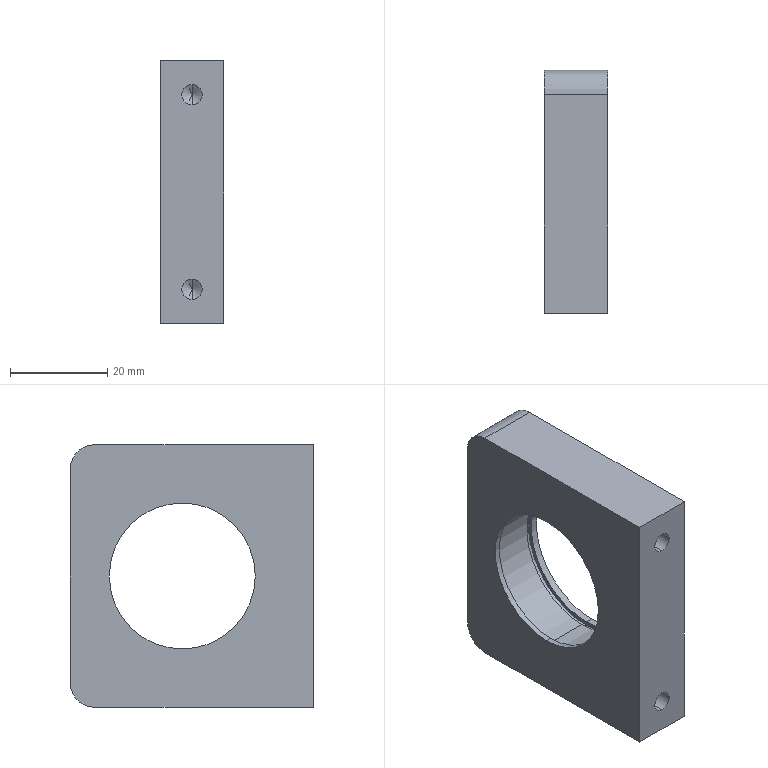Part | SolidWorks | features ICE 4, 3DProfileFeature 2, HoleWzd 2, ExtruThin 1, Fillet 1, RevCut 1 | 1 solid | 35 faces | box 13 x 50 x 54 mm | volume 23974 mm3 | cylinder 18 | plane 9 | cone 8 | commonest cylinder face diameters 3.3 x4 4.2 x4 32 x4 10 x2 30 x2 33.7 x2
STEP:
#1=CARTESIAN_POINT('',(-6.5,39.9,-16.65));
#2=VERTEX_POINT('',#1);
#3=CARTESIAN_POINT('',(-6.5,39.9,-13.35));
#4=VERTEX_POINT('',#3);
#5=CARTESIAN_POINT('',(-6.5,39.9,-15.));
#6=DIRECTION('',(0.,1.,0.));
#7=DIRECTION('',(0.,0.,1.));
#8=AXIS2_PLACEMENT_3D('',#5,#6,#7);
#9=CIRCLE('',#8,1.65);
#10=EDGE_CURVE('',#2,#4,#9,.T.);
#11=ORIENTED_EDGE('',*,*,#10,.F.);
#12=CARTESIAN_POINT('',(-6.5,50.,-16.65));
#13=VERTEX_POINT('',#12);
#14=CARTESIAN_POINT('',(-6.5,50.,-16.65));
#15=DIRECTION('',(0.,1.,0.));
#16=VECTOR('',#15,1000.);
#17=LINE('',#14,#16);
#18=EDGE_CURVE('',#2,#13,#17,.T.);
#19=ORIENTED_EDGE('',*,*,#18,.T.);
#20=CARTESIAN_POINT('',(-6.5,50.,-13.35));
#21=VERTEX_POINT('',#20);
#22=CARTESIAN_POINT('',(-6.5,50.,-15.));
#23=DIRECTION('',(0.,1.,0.));
#24=DIRECTION('',(0.,0.,1.));
#25=AXIS2_PLACEMENT_3D('',#22,#23,#24);
#26=CIRCLE('',#25,1.65);
#27=EDGE_CURVE('',#13,#21,#26,.T.);
#28=ORIENTED_EDGE('',*,*,#27,.T.);
#29=CARTESIAN_POINT('',(-6.5,50.,-13.35));
#30=DIRECTION('',(0.,1.,0.));
#31=VECTOR('',#30,1000.);
#32=LINE('',#29,#31);
#33=EDGE_CURVE('',#4,#21,#32,.T.);
#34=ORIENTED_EDGE('',*,*,#33,.F.);
#35=EDGE_LOOP('',(#11,#19,#28,#34));
#36=FACE_OUTER_BOUND('',#35,.T.);
#37=CARTESIAN_POINT('',(-6.5,50.,-15.));
#38=DIRECTION('',(0.,1.,0.));
#39=DIRECTION('',(0.,0.,1.));
#40=AXIS2_PLACEMENT_3D('',#37,#38,#39);
#41=CYLINDRICAL_SURFACE('',#40,1.65);
#42=ADVANCED_FACE('',(#36),#41,.F.);
#43=CARTESIAN_POINT('',(-6.5,38.909,-15.));
#44=VERTEX_POINT('',#43);
#45=CARTESIAN_POINT('',(-6.5,39.9,-13.35));
#46=DIRECTION('',(0.,0.515,0.8572));
#47=VECTOR('',#46,1000.);
#48=LINE('',#45,#47);
#49=EDGE_CURVE('',#44,#4,#48,.T.);
#50=ORIENTED_EDGE('',*,*,#49,.F.);
#51=CARTESIAN_POINT('',(-6.5,39.9,-16.65));
#52=DIRECTION('',(0.,0.515,-0.8572));
#53=VECTOR('',#52,1000.);
#54=LINE('',#51,#53);
#55=EDGE_CURVE('',#44,#2,#54,.T.);
#56=ORIENTED_EDGE('',*,*,#55,.T.);
#57=ORIENTED_EDGE('',*,*,#10,.T.);
#58=EDGE_LOOP('',(#50,#56,#57));
#59=FACE_OUTER_BOUND('',#58,.T.);
#60=CARTESIAN_POINT('',(-6.5,39.9,-15.));
#61=DIRECTION('',(0.,1.,0.));
#62=DIRECTION('',(0.,0.,1.));
#63=AXIS2_PLACEMENT_3D('',#60,#61,#62);
#64=CONICAL_SURFACE('',#63,1.65,1.03);
#65=ADVANCED_FACE('',(#59),#64,.F.);
#66=CARTESIAN_POINT('',(-6.5,39.9,13.35));
#67=VERTEX_POINT('',#66);
#68=CARTESIAN_POINT('',(-6.5,39.9,16.65));
#69=VERTEX_POINT('',#68);
#70=CARTESIAN_POINT('',(-6.5,39.9,15.));
#71=DIRECTION('',(0.,1.,0.));
#72=DIRECTION('',(0.,0.,1.));
#73=AXIS2_PLACEMENT_3D('',#70,#71,#72);
#74=CIRCLE('',#73,1.65);
#75=EDGE_CURVE('',#67,#69,#74,.T.);
#76=ORIENTED_EDGE('',*,*,#75,.F.);
#77=CARTESIAN_POINT('',(-6.5,50.,13.35));
#78=VERTEX_POINT('',#77);
#79=CARTESIAN_POINT('',(-6.5,50.,13.35));
#80=DIRECTION('',(0.,1.,0.));
#81=VECTOR('',#80,1000.);
#82=LINE('',#79,#81);
#83=EDGE_CURVE('',#67,#78,#82,.T.);
#84=ORIENTED_EDGE('',*,*,#83,.T.);
#85=CARTESIAN_POINT('',(-6.5,50.,16.65));
#86=VERTEX_POINT('',#85);
#87=CARTESIAN_POINT('',(-6.5,50.,15.));
#88=DIRECTION('',(0.,1.,0.));
#89=DIRECTION('',(0.,0.,1.));
#90=AXIS2_PLACEMENT_3D('',#87,#88,#89);
#91=CIRCLE('',#90,1.65);
#92=EDGE_CURVE('',#78,#86,#91,.T.);
#93=ORIENTED_EDGE('',*,*,#92,.T.);
#94=CARTESIAN_POINT('',(-6.5,50.,16.65));
#95=DIRECTION('',(0.,1.,0.));
#96=VECTOR('',#95,1000.);
#97=LINE('',#94,#96);
#98=EDGE_CURVE('',#69,#86,#97,.T.);
#99=ORIENTED_EDGE('',*,*,#98,.F.);
#100=EDGE_LOOP('',(#76,#84,#93,#99));
#101=FACE_OUTER_BOUND('',#100,.T.);
#102=CARTESIAN_POINT('',(-6.5,50.,15.));
#103=DIRECTION('',(0.,1.,0.));
#104=DIRECTION('',(0.,0.,1.));
#105=AXIS2_PLACEMENT_3D('',#102,#103,#104);
#106=CYLINDRICAL_SURFACE('',#105,1.65);
#107=ADVANCED_FACE('',(#101),#106,.F.);
#108=CARTESIAN_POINT('',(-6.5,38.909,15.));
#109=VERTEX_POINT('',#108);
#110=CARTESIAN_POINT('',(-6.5,39.9,16.65));
#111=DIRECTION('',(0.,0.515,0.8572));
#112=VECTOR('',#111,1000.);
#113=LINE('',#110,#112);
#114=EDGE_CURVE('',#109,#69,#113,.T.);
#115=ORIENTED_EDGE('',*,*,#114,.F.);
#116=CARTESIAN_POINT('',(-6.5,39.9,13.35));
#117=DIRECTION('',(0.,0.515,-0.8572));
#118=VECTOR('',#117,1000.);
#119=LINE('',#116,#118);
#120=EDGE_CURVE('',#109,#67,#119,.T.);
#121=ORIENTED_EDGE('',*,*,#120,.T.);
#122=ORIENTED_EDGE('',*,*,#75,.T.);
#123=EDGE_LOOP('',(#115,#121,#122));
#124=FACE_OUTER_BOUND('',#123,.T.);
#125=CARTESIAN_POINT('',(-6.5,39.9,15.));
#126=DIRECTION('',(0.,1.,0.));
#127=DIRECTION('',(0.,0.,1.));
#128=AXIS2_PLACEMENT_3D('',#125,#126,#127);
#129=CONICAL_SURFACE('',#128,1.65,1.03);
#130=ADVANCED_FACE('',(#124),#129,.F.);
#131=CARTESIAN_POINT('',(-6.5,12.4,22.1));
#132=VERTEX_POINT('',#131);
#133=CARTESIAN_POINT('',(-6.5,12.4,17.9));
#134=VERTEX_POINT('',#133);
#135=CARTESIAN_POINT('',(-6.5,12.4,20.));
#136=DIRECTION('',(0.,-1.,0.));
#137=DIRECTION('',(0.,0.,-1.));
#138=AXIS2_PLACEMENT_3D('',#135,#136,#137);
#139=CIRCLE('',#138,2.1);
#140=EDGE_CURVE('',#132,#134,#139,.T.);
#141=ORIENTED_EDGE('',*,*,#140,.F.);
#142=CARTESIAN_POINT('',(-6.5,0.,22.1));
#143=VERTEX_POINT('',#142);
#144=CARTESIAN_POINT('',(-6.5,0.,22.1));
#145=DIRECTION('',(0.,-1.,0.));
#146=VECTOR('',#145,1000.);
#147=LINE('',#144,#146);
#148=EDGE_CURVE('',#132,#143,#147,.T.);
#149=ORIENTED_EDGE('',*,*,#148,.T.);
#150=CARTESIAN_POINT('',(-6.5,0.,17.9));
#151=VERTEX_POINT('',#150);
#152=CARTESIAN_POINT('',(-6.5,0.,20.));
#153=DIRECTION('',(0.,-1.,0.));
#154=DIRECTION('',(0.,0.,-1.));
#155=AXIS2_PLACEMENT_3D('',#152,#153,#154);
#156=CIRCLE('',#155,2.1);
#157=EDGE_CURVE('',#143,#151,#156,.T.);
#158=ORIENTED_EDGE('',*,*,#157,.T.);
#159=CARTESIAN_POINT('',(-6.5,0.,17.9));
#160=DIRECTION('',(0.,-1.,0.));
#161=VECTOR('',#160,1000.);
#162=LINE('',#159,#161);
#163=EDGE_CURVE('',#134,#151,#162,.T.);
#164=ORIENTED_EDGE('',*,*,#163,.F.);
#165=EDGE_LOOP('',(#141,#149,#158,#164));
#166=FACE_OUTER_BOUND('',#165,.T.);
#167=CARTESIAN_POINT('',(-6.5,0.,20.));
#168=DIRECTION('',(0.,-1.,0.));
#169=DIRECTION('',(0.,0.,-1.));
#170=AXIS2_PLACEMENT_3D('',#167,#168,#169);
#171=CYLINDRICAL_SURFACE('',#170,2.1);
#172=ADVANCED_FACE('',(#166),#171,.F.);
#173=CARTESIAN_POINT('',(-6.5,13.662,20.));
#174=VERTEX_POINT('',#173);
#175=CARTESIAN_POINT('',(-6.5,12.4,17.9));
#176=DIRECTION('',(0.,-0.515,-0.8572));
#177=VECTOR('',#176,1000.);
#178=LINE('',#175,#177);
#179=EDGE_CURVE('',#174,#134,#178,.T.);
#180=ORIENTED_EDGE('',*,*,#179,.F.);
#181=CARTESIAN_POINT('',(-6.5,12.4,22.1));
#182=DIRECTION('',(0.,-0.515,0.8572));
#183=VECTOR('',#182,1000.);
#184=LINE('',#181,#183);
#185=EDGE_CURVE('',#174,#132,#184,.T.);
#186=ORIENTED_EDGE('',*,*,#185,.T.);
#187=ORIENTED_EDGE('',*,*,#140,.T.);
#188=EDGE_LOOP('',(#180,#186,#187));
#189=FACE_OUTER_BOUND('',#188,.T.);
#190=CARTESIAN_POINT('',(-6.5,12.4,20.));
#191=DIRECTION('',(0.,-1.,0.));
#192=DIRECTION('',(0.,0.,-1.));
#193=AXIS2_PLACEMENT_3D('',#190,#191,#192);
#194=CONICAL_SURFACE('',#193,2.1,1.03);
#195=ADVANCED_FACE('',(#189),#194,.F.);
#196=CARTESIAN_POINT('',(-6.5,12.4,-17.9));
#197=VERTEX_POINT('',#196);
#198=CARTESIAN_POINT('',(-6.5,12.4,-22.1));
#199=VERTEX_POINT('',#198);
#200=CARTESIAN_POINT('',(-6.5,12.4,-20.));
#201=DIRECTION('',(0.,-1.,0.));
#202=DIRECTION('',(0.,0.,-1.));
#203=AXIS2_PLACEMENT_3D('',#200,#201,#202);
#204=CIRCLE('',#203,2.1);
#205=EDGE_CURVE('',#197,#199,#204,.T.);
#206=ORIENTED_EDGE('',*,*,#205,.F.);
#207=CARTESIAN_POINT('',(-6.5,0.,-17.9));
#208=VERTEX_POINT('',#207);
#209=CARTESIAN_POINT('',(-6.5,0.,-17.9));
#210=DIRECTION('',(0.,-1.,0.));
#211=VECTOR('',#210,1000.);
#212=LINE('',#209,#211);
#213=EDGE_CURVE('',#197,#208,#212,.T.);
#214=ORIENTED_EDGE('',*,*,#213,.T.);
#215=CARTESIAN_POINT('',(-6.5,0.,-22.1));
#216=VERTEX_POINT('',#215);
#217=CARTESIAN_POINT('',(-6.5,0.,-20.));
#218=DIRECTION('',(0.,-1.,0.));
#219=DIRECTION('',(0.,0.,-1.));
#220=AXIS2_PLACEMENT_3D('',#217,#218,#219);
#221=CIRCLE('',#220,2.1);
#222=EDGE_CURVE('',#208,#216,#221,.T.);
#223=ORIENTED_EDGE('',*,*,#222,.T.);
#224=CARTESIAN_POINT('',(-6.5,0.,-22.1));
#225=DIRECTION('',(0.,-1.,0.));
#226=VECTOR('',#225,1000.);
#227=LINE('',#224,#226);
#228=EDGE_CURVE('',#199,#216,#227,.T.);
#229=ORIENTED_EDGE('',*,*,#228,.F.);
#230=EDGE_LOOP('',(#206,#214,#223,#229));
#231=FACE_OUTER_BOUND('',#230,.T.);
#232=CARTESIAN_POINT('',(-6.5,0.,-20.));
#233=DIRECTION('',(0.,-1.,0.));
#234=DIRECTION('',(0.,0.,-1.));
#235=AXIS2_PLACEMENT_3D('',#232,#233,#234);
#236=CYLINDRICAL_SURFACE('',#235,2.1);
#237=ADVANCED_FACE('',(#231),#236,.F.);
#238=CARTESIAN_POINT('',(-6.5,13.662,-20.));
#239=VERTEX_POINT('',#238);
#240=CARTESIAN_POINT('',(-6.5,12.4,-22.1));
#241=DIRECTION('',(0.,-0.515,-0.8572));
#242=VECTOR('',#241,1000.);
#243=LINE('',#240,#242);
#244=EDGE_CURVE('',#239,#199,#243,.T.);
#245=ORIENTED_EDGE('',*,*,#244,.F.);
#246=CARTESIAN_POINT('',(-6.5,12.4,-17.9));
#247=DIRECTION('',(0.,-0.515,0.8572));
#248=VECTOR('',#247,1000.);
#249=LINE('',#246,#248);
#250=EDGE_CURVE('',#239,#197,#249,.T.);
#251=ORIENTED_EDGE('',*,*,#250,.T.);
#252=ORIENTED_EDGE('',*,*,#205,.T.);
#253=EDGE_LOOP('',(#245,#251,#252));
#254=FACE_OUTER_BOUND('',#253,.T.);
#255=CARTESIAN_POINT('',(-6.5,12.4,-20.));
#256=DIRECTION('',(0.,-1.,0.));
#257=DIRECTION('',(0.,0.,-1.));
#258=AXIS2_PLACEMENT_3D('',#255,#256,#257);
#259=CONICAL_SURFACE('',#258,2.1,1.03);
#260=ADVANCED_FACE('',(#254),#259,.F.);
#261=CARTESIAN_POINT('',(-1.5,27.,-16.85));
#262=VERTEX_POINT('',#261);
#263=CARTESIAN_POINT('',(-1.5,27.,16.85));
#264=VERTEX_POINT('',#263);
#265=CARTESIAN_POINT('',(-1.5,27.,0.));
#266=DIRECTION('',(-1.,0.,0.));
#267=DIRECTION('',(0.,0.,1.));
#268=AXIS2_PLACEMENT_3D('',#265,#266,#267);
#269=CIRCLE('',#268,16.85);
#270=EDGE_CURVE('',#262,#264,#269,.T.);
#271=ORIENTED_EDGE('',*,*,#270,.F.);
#272=CARTESIAN_POINT('',(-2.8,27.,-16.85));
#273=VERTEX_POINT('',#272);
#274=CARTESIAN_POINT('',(-11.8,27.,-16.85));
#275=DIRECTION('',(-1.,0.,0.));
#276=VECTOR('',#275,1000.);
#277=LINE('',#274,#276);
#278=EDGE_CURVE('',#262,#273,#277,.T.);
#279=ORIENTED_EDGE('',*,*,#278,.T.);
#280=CARTESIAN_POINT('',(-2.8,27.,16.85));
#281=VERTEX_POINT('',#280);
#282=CARTESIAN_POINT('',(-2.8,27.,0.));
#283=DIRECTION('',(-1.,0.,0.));
#284=DIRECTION('',(0.,0.,1.));
#285=AXIS2_PLACEMENT_3D('',#282,#283,#284);
#286=CIRCLE('',#285,16.85);
#287=EDGE_CURVE('',#273,#281,#286,.T.);
#288=ORIENTED_EDGE('',*,*,#287,.T.);
#289=CARTESIAN_POINT('',(-11.8,27.,16.85));
#290=DIRECTION('',(-1.,0.,0.));
#291=VECTOR('',#290,1000.);
#292=LINE('',#289,#291);
#293=EDGE_CURVE('',#264,#281,#292,.T.);
#294=ORIENTED_EDGE('',*,*,#293,.F.);
#295=EDGE_LOOP('',(#271,#279,#288,#294));
#296=FACE_OUTER_BOUND('',#295,.T.);
#297=CARTESIAN_POINT('',(-11.8,27.,0.));
#298=DIRECTION('',(-1.,0.,0.));
#299=DIRECTION('',(0.,0.,1.));
#300=AXIS2_PLACEMENT_3D('',#297,#298,#299);
#301=CYLINDRICAL_SURFACE('',#300,16.85);
#302=ADVANCED_FACE('',(#296),#301,.F.);
#303=CARTESIAN_POINT('',(-11.8,27.,-15.));
#304=VERTEX_POINT('',#303);
#305=CARTESIAN_POINT('',(-11.8,27.,15.));
#306=VERTEX_POINT('',#305);
#307=CARTESIAN_POINT('',(-11.8,27.,0.));
#308=DIRECTION('',(-1.,0.,0.));
#309=DIRECTION('',(0.,0.,1.));
#310=AXIS2_PLACEMENT_3D('',#307,#308,#309);
#311=CIRCLE('',#310,15.);
#312=EDGE_CURVE('',#304,#306,#311,.T.);
#313=ORIENTED_EDGE('',*,*,#312,.F.);
#314=CARTESIAN_POINT('',(-13.,27.,-15.));
#315=VERTEX_POINT('',#314);
#316=CARTESIAN_POINT('',(-11.8,27.,-15.));
#317=DIRECTION('',(-1.,0.,0.));
#318=VECTOR('',#317,1000.);
#319=LINE('',#316,#318);
#320=EDGE_CURVE('',#304,#315,#319,.T.);
#321=ORIENTED_EDGE('',*,*,#320,.T.);
#322=CARTESIAN_POINT('',(-13.,27.,15.));
#323=VERTEX_POINT('',#322);
#324=CARTESIAN_POINT('',(-13.,27.,0.));
#325=DIRECTION('',(-1.,0.,0.));
#326=DIRECTION('',(0.,0.,1.));
#327=AXIS2_PLACEMENT_3D('',#324,#325,#326);
#328=CIRCLE('',#327,15.);
#329=EDGE_CURVE('',#315,#323,#328,.T.);
#330=ORIENTED_EDGE('',*,*,#329,.T.);
#331=CARTESIAN_POINT('',(-11.8,27.,15.));
#332=DIRECTION('',(-1.,0.,0.));
#333=VECTOR('',#332,1000.);
#334=LINE('',#331,#333);
#335=EDGE_CURVE('',#306,#323,#334,.T.);
#336=ORIENTED_EDGE('',*,*,#335,.F.);
#337=EDGE_LOOP('',(#313,#321,#330,#336));
#338=FACE_OUTER_BOUND('',#337,.T.);
#339=CARTESIAN_POINT('',(-11.8,27.,0.));
#340=DIRECTION('',(-1.,0.,0.));
#341=DIRECTION('',(0.,0.,1.));
#342=AXIS2_PLACEMENT_3D('',#339,#340,#341);
#343=CYLINDRICAL_SURFACE('',#342,15.);
#344=ADVANCED_FACE('',(#338),#343,.F.);
#345=CARTESIAN_POINT('',(-1.5,27.,-16.));
#346=VERTEX_POINT('',#345);
#347=CARTESIAN_POINT('',(-1.5,27.,16.));
#348=VERTEX_POINT('',#347);
#349=CARTESIAN_POINT('',(-1.5,27.,0.));
#350=DIRECTION('',(-1.,0.,0.));
#351=DIRECTION('',(0.,0.,1.));
#352=AXIS2_PLACEMENT_3D('',#349,#350,#351);
#353=CIRCLE('',#352,16.);
#354=EDGE_CURVE('',#346,#348,#353,.T.);
#355=ORIENTED_EDGE('',*,*,#354,.T.);
#356=CARTESIAN_POINT('',(0.,27.,16.));
#357=VERTEX_POINT('',#356);
#358=CARTESIAN_POINT('',(-13.,27.,16.));
#359=DIRECTION('',(1.,0.,0.));
#360=VECTOR('',#359,1000.);
#361=LINE('',#358,#360);
#362=EDGE_CURVE('',#348,#357,#361,.T.);
#363=ORIENTED_EDGE('',*,*,#362,.T.);
#364=CARTESIAN_POINT('',(0.,27.,-16.));
#365=VERTEX_POINT('',#364);
#366=CARTESIAN_POINT('',(0.,27.,0.));
#367=DIRECTION('',(1.,0.,0.));
#368=DIRECTION('',(0.,0.,-1.));
#369=AXIS2_PLACEMENT_3D('',#366,#367,#368);
#370=CIRCLE('',#369,16.);
#371=EDGE_CURVE('',#357,#365,#370,.T.);
#372=ORIENTED_EDGE('',*,*,#371,.T.);
#373=CARTESIAN_POINT('',(-13.,27.,-16.));
#374=DIRECTION('',(1.,0.,0.));
#375=VECTOR('',#374,1000.);
#376=LINE('',#373,#375);
#377=EDGE_CURVE('',#346,#365,#376,.T.);
#378=ORIENTED_EDGE('',*,*,#377,.F.);
#379=EDGE_LOOP('',(#355,#363,#372,#378));
#380=FACE_OUTER_BOUND('',#379,.T.);
#381=CARTESIAN_POINT('',(-13.,27.,0.));
#382=DIRECTION('',(1.,0.,0.));
#383=DIRECTION('',(0.,0.,-1.));
#384=AXIS2_PLACEMENT_3D('',#381,#382,#383);
#385=CYLINDRICAL_SURFACE('',#384,16.);
#386=ADVANCED_FACE('',(#380),#385,.F.);
#387=CARTESIAN_POINT('',(-11.8,27.,16.));
#388=VERTEX_POINT('',#387);
#389=CARTESIAN_POINT('',(-11.8,27.,-16.));
#390=VERTEX_POINT('',#389);
#391=CARTESIAN_POINT('',(-11.8,27.,0.));
#392=DIRECTION('',(1.,0.,0.));
#393=DIRECTION('',(0.,0.,1.));
#394=AXIS2_PLACEMENT_3D('',#391,#392,#393);
#395=CIRCLE('',#394,16.);
#396=EDGE_CURVE('',#388,#390,#395,.T.);
#397=ORIENTED_EDGE('',*,*,#396,.F.);
#398=CARTESIAN_POINT('',(-2.8,27.,16.));
#399=VERTEX_POINT('',#398);
#400=CARTESIAN_POINT('',(-13.,27.,16.));
#401=DIRECTION('',(1.,0.,0.));
#402=VECTOR('',#401,1000.);
#403=LINE('',#400,#402);
#404=EDGE_CURVE('',#388,#399,#403,.T.);
#405=ORIENTED_EDGE('',*,*,#404,.T.);
#406=CARTESIAN_POINT('',(-2.8,27.,-16.));
#407=VERTEX_POINT('',#406);
#408=CARTESIAN_POINT('',(-2.8,27.,0.));
#409=DIRECTION('',(-1.,0.,0.));
#410=DIRECTION('',(0.,0.,1.));
#411=AXIS2_PLACEMENT_3D('',#408,#409,#410);
#412=CIRCLE('',#411,16.);
#413=EDGE_CURVE('',#407,#399,#412,.T.);
#414=ORIENTED_EDGE('',*,*,#413,.F.);
#415=CARTESIAN_POINT('',(-13.,27.,-16.));
#416=DIRECTION('',(1.,0.,0.));
#417=VECTOR('',#416,1000.);
#418=LINE('',#415,#417);
#419=EDGE_CURVE('',#390,#407,#418,.T.);
#420=ORIENTED_EDGE('',*,*,#419,.F.);
#421=EDGE_LOOP('',(#397,#405,#414,#420));
#422=FACE_OUTER_BOUND('',#421,.T.);
#423=CARTESIAN_POINT('',(-13.,27.,0.));
#424=DIRECTION('',(1.,0.,0.));
#425=DIRECTION('',(0.,0.,-1.));
#426=AXIS2_PLACEMENT_3D('',#423,#424,#425);
#427=CYLINDRICAL_SURFACE('',#426,16.);
#428=ADVANCED_FACE('',(#422),#427,.F.);
#429=CARTESIAN_POINT('',(-13.,27.,0.));
#430=DIRECTION('',(-1.,0.,0.));
#431=DIRECTION('',(0.,0.,1.));
#432=AXIS2_PLACEMENT_3D('',#429,#430,#431);
#433=CIRCLE('',#432,15.);
#434=EDGE_CURVE('',#323,#315,#433,.T.);
#435=ORIENTED_EDGE('',*,*,#434,.F.);
#436=ORIENTED_EDGE('',*,*,#329,.F.);
#437=EDGE_LOOP('',(#435,#436));
#438=FACE_BOUND('',#437,.T.);
#439=CARTESIAN_POINT('',(-13.,0.,27.));
#440=VERTEX_POINT('',#439);
#441=CARTESIAN_POINT('',(-13.,0.,-27.));
#442=VERTEX_POINT('',#441);
#443=CARTESIAN_POINT('',(-13.,0.,47.5));
#444=DIRECTION('',(0.,0.,-1.));
#445=VECTOR('',#444,1000.);
#446=LINE('',#443,#445);
#447=EDGE_CURVE('',#440,#442,#446,.T.);
#448=ORIENTED_EDGE('',*,*,#447,.F.);
#449=CARTESIAN_POINT('',(-13.,45.,27.));
#450=VERTEX_POINT('',#449);
#451=CARTESIAN_POINT('',(-13.,0.,27.));
#452=DIRECTION('',(0.,-1.,0.));
#453=VECTOR('',#452,1000.);
#454=LINE('',#451,#453);
#455=EDGE_CURVE('',#450,#440,#454,.T.);
#456=ORIENTED_EDGE('',*,*,#455,.F.);
#457=CARTESIAN_POINT('',(-13.,50.,22.));
#458=VERTEX_POINT('',#457);
#459=CARTESIAN_POINT('',(-13.,45.,22.));
#460=DIRECTION('',(-1.,0.,0.));
#461=DIRECTION('',(0.,0.,-1.));
#462=AXIS2_PLACEMENT_3D('',#459,#460,#461);
#463=CIRCLE('',#462,5.);
#464=EDGE_CURVE('',#450,#458,#463,.T.);
#465=ORIENTED_EDGE('',*,*,#464,.T.);
#466=CARTESIAN_POINT('',(-13.,50.,-22.));
#467=VERTEX_POINT('',#466);
#468=CARTESIAN_POINT('',(-13.,50.,27.));
#469=DIRECTION('',(0.,0.,-1.));
#470=VECTOR('',#469,1000.);
#471=LINE('',#468,#470);
#472=EDGE_CURVE('',#458,#467,#471,.T.);
#473=ORIENTED_EDGE('',*,*,#472,.T.);
#474=CARTESIAN_POINT('',(-13.,45.,-27.));
#475=VERTEX_POINT('',#474);
#476=CARTESIAN_POINT('',(-13.,45.,-22.));
#477=DIRECTION('',(-1.,0.,0.));
#478=DIRECTION('',(0.,0.,-1.));
#479=AXIS2_PLACEMENT_3D('',#476,#477,#478);
#480=CIRCLE('',#479,5.);
#481=EDGE_CURVE('',#467,#475,#480,.T.);
#482=ORIENTED_EDGE('',*,*,#481,.T.);
#483=CARTESIAN_POINT('',(-13.,0.,-27.));
#484=DIRECTION('',(0.,-1.,0.));
#485=VECTOR('',#484,1000.);
#486=LINE('',#483,#485);
#487=EDGE_CURVE('',#475,#442,#486,.T.);
#488=ORIENTED_EDGE('',*,*,#487,.T.);
#489=EDGE_LOOP('',(#448,#456,#465,#473,#482,#488));
#490=FACE_OUTER_BOUND('',#489,.T.);
#491=CARTESIAN_POINT('',(-13.,0.,27.));
#492=DIRECTION('',(1.,0.,0.));
#493=DIRECTION('',(0.,0.,-1.));
#494=AXIS2_PLACEMENT_3D('',#491,#492,#493);
#495=PLANE('',#494);
#496=ADVANCED_FACE('',(#438,#490),#495,.F.);
#497=CARTESIAN_POINT('',(0.,45.,27.));
#498=VERTEX_POINT('',#497);
#499=CARTESIAN_POINT('',(0.,0.,27.));
#500=VERTEX_POINT('',#499);
#501=CARTESIAN_POINT('',(0.,0.,27.));
#502=DIRECTION('',(0.,-1.,0.));
#503=VECTOR('',#502,1000.);
#504=LINE('',#501,#503);
#505=EDGE_CURVE('',#498,#500,#504,.T.);
#506=ORIENTED_EDGE('',*,*,#505,.F.);
#507=CARTESIAN_POINT('',(-13.,45.,27.));
#508=DIRECTION('',(-1.,0.,0.));
#509=VECTOR('',#508,1000.);
#510=LINE('',#507,#509);
#511=EDGE_CURVE('',#498,#450,#510,.T.);
#512=ORIENTED_EDGE('',*,*,#511,.T.);
#513=ORIENTED_EDGE('',*,*,#455,.T.);
#514=CARTESIAN_POINT('',(0.,0.,27.));
#515=DIRECTION('',(-1.,0.,0.));
#516=VECTOR('',#515,1000.);
#517=LINE('',#514,#516);
#518=EDGE_CURVE('',#500,#440,#517,.T.);
#519=ORIENTED_EDGE('',*,*,#518,.F.);
#520=EDGE_LOOP('',(#506,#512,#513,#519));
#521=FACE_OUTER_BOUND('',#520,.T.);
#522=CARTESIAN_POINT('',(0.,0.,27.));
#523=DIRECTION('',(0.,0.,-1.));
#524=DIRECTION('',(-1.,0.,0.));
#525=AXIS2_PLACEMENT_3D('',#522,#523,#524);
#526=PLANE('',#525);
#527=ADVANCED_FACE('',(#521),#526,.F.);
#528=ORIENTED_EDGE('',*,*,#487,.F.);
#529=CARTESIAN_POINT('',(0.,45.,-27.));
#530=VERTEX_POINT('',#529);
#531=CARTESIAN_POINT('',(0.,45.,-27.));
#532=DIRECTION('',(1.,0.,0.));
#533=VECTOR('',#532,1000.);
#534=LINE('',#531,#533);
#535=EDGE_CURVE('',#475,#530,#534,.T.);
#536=ORIENTED_EDGE('',*,*,#535,.T.);
#537=CARTESIAN_POINT('',(0.,0.,-27.));
#538=VERTEX_POINT('',#537);
#539=CARTESIAN_POINT('',(0.,0.,-27.));
#540=DIRECTION('',(0.,-1.,0.));
#541=VECTOR('',#540,1000.);
#542=LINE('',#539,#541);
#543=EDGE_CURVE('',#530,#538,#542,.T.);
#544=ORIENTED_EDGE('',*,*,#543,.T.);
#545=CARTESIAN_POINT('',(0.,0.,-27.));
#546=DIRECTION('',(-1.,0.,0.));
#547=VECTOR('',#546,1000.);
#548=LINE('',#545,#547);
#549=EDGE_CURVE('',#538,#442,#548,.T.);
#550=ORIENTED_EDGE('',*,*,#549,.T.);
#551=EDGE_LOOP('',(#528,#536,#544,#550));
#552=FACE_OUTER_BOUND('',#551,.T.);
#553=CARTESIAN_POINT('',(0.,0.,-27.));
#554=DIRECTION('',(0.,0.,-1.));
#555=DIRECTION('',(-1.,0.,0.));
#556=AXIS2_PLACEMENT_3D('',#553,#554,#555);
#557=PLANE('',#556);
#558=ADVANCED_FACE('',(#552),#557,.T.);
#559=ORIENTED_EDGE('',*,*,#404,.F.);
#560=CARTESIAN_POINT('',(-11.8,27.,0.));
#561=DIRECTION('',(1.,0.,0.));
#562=DIRECTION('',(0.,0.,1.));
#563=AXIS2_PLACEMENT_3D('',#560,#561,#562);
#564=CIRCLE('',#563,16.);
#565=EDGE_CURVE('',#390,#388,#564,.T.);
#566=ORIENTED_EDGE('',*,*,#565,.F.);
#567=ORIENTED_EDGE('',*,*,#419,.T.);
#568=CARTESIAN_POINT('',(-2.8,27.,0.));
#569=DIRECTION('',(-1.,0.,0.));
#570=DIRECTION('',(0.,0.,1.));
#571=AXIS2_PLACEMENT_3D('',#568,#569,#570);
#572=CIRCLE('',#571,16.);
#573=EDGE_CURVE('',#399,#407,#572,.T.);
#574=ORIENTED_EDGE('',*,*,#573,.F.);
#575=EDGE_LOOP('',(#559,#566,#567,#574));
#576=FACE_OUTER_BOUND('',#575,.T.);
#577=CARTESIAN_POINT('',(-13.,27.,0.));
#578=DIRECTION('',(1.,0.,0.));
#579=DIRECTION('',(0.,0.,-1.));
#580=AXIS2_PLACEMENT_3D('',#577,#578,#579);
#581=CYLINDRICAL_SURFACE('',#580,16.);
#582=ADVANCED_FACE('',(#576),#581,.F.);
#583=ORIENTED_EDGE('',*,*,#362,.F.);
#584=CARTESIAN_POINT('',(-1.5,27.,0.));
#585=DIRECTION('',(-1.,0.,0.));
#586=DIRECTION('',(0.,0.,1.));
#587=AXIS2_PLACEMENT_3D('',#584,#585,#586);
#588=CIRCLE('',#587,16.);
#589=EDGE_CURVE('',#348,#346,#588,.T.);
#590=ORIENTED_EDGE('',*,*,#589,.T.);
#591=ORIENTED_EDGE('',*,*,#377,.T.);
#592=CARTESIAN_POINT('',(0.,27.,0.));
#593=DIRECTION('',(1.,0.,0.));
#594=DIRECTION('',(0.,0.,-1.));
#595=AXIS2_PLACEMENT_3D('',#592,#593,#594);
#596=CIRCLE('',#595,16.);
#597=EDGE_CURVE('',#365,#357,#596,.T.);
#598=ORIENTED_EDGE('',*,*,#597,.T.);
#599=EDGE_LOOP('',(#583,#590,#591,#598));
#600=FACE_OUTER_BOUND('',#599,.T.);
#601=CARTESIAN_POINT('',(-13.,27.,0.));
#602=DIRECTION('',(1.,0.,0.));
#603=DIRECTION('',(0.,0.,-1.));
#604=AXIS2_PLACEMENT_3D('',#601,#602,#603);
#605=CYLINDRICAL_SURFACE('',#604,16.);
#606=ADVANCED_FACE('',(#600),#605,.F.);
#607=ORIENTED_EDGE('',*,*,#597,.F.);
#608=ORIENTED_EDGE('',*,*,#371,.F.);
#609=EDGE_LOOP('',(#607,#608));
#610=FACE_BOUND('',#609,.T.);
#611=ORIENTED_EDGE('',*,*,#543,.F.);
#612=CARTESIAN_POINT('',(0.,50.,-22.));
#613=VERTEX_POINT('',#612);
#614=CARTESIAN_POINT('',(0.,45.,-22.));
#615=DIRECTION('',(1.,0.,0.));
#616=DIRECTION('',(0.,0.,-1.));
#617=AXIS2_PLACEMENT_3D('',#614,#615,#616);
#618=CIRCLE('',#617,5.);
#619=EDGE_CURVE('',#530,#613,#618,.T.);
#620=ORIENTED_EDGE('',*,*,#619,.T.);
#621=CARTESIAN_POINT('',(0.,50.,22.));
#622=VERTEX_POINT('',#621);
#623=CARTESIAN_POINT('',(0.,50.,27.));
#624=DIRECTION('',(0.,0.,-1.));
#625=VECTOR('',#624,1000.);
#626=LINE('',#623,#625);
#627=EDGE_CURVE('',#622,#613,#626,.T.);
#628=ORIENTED_EDGE('',*,*,#627,.F.);
#629=CARTESIAN_POINT('',(0.,45.,22.));
#630=DIRECTION('',(1.,0.,0.));
#631=DIRECTION('',(0.,0.,-1.));
#632=AXIS2_PLACEMENT_3D('',#629,#630,#631);
#633=CIRCLE('',#632,5.);
#634=EDGE_CURVE('',#622,#498,#633,.T.);
#635=ORIENTED_EDGE('',*,*,#634,.T.);
#636=ORIENTED_EDGE('',*,*,#505,.T.);
#637=CARTESIAN_POINT('',(0.,0.,27.));
#638=DIRECTION('',(0.,0.,-1.));
#639=VECTOR('',#638,1000.);
#640=LINE('',#637,#639);
#641=EDGE_CURVE('',#500,#538,#640,.T.);
#642=ORIENTED_EDGE('',*,*,#641,.T.);
#643=EDGE_LOOP('',(#611,#620,#628,#635,#636,#642));
#644=FACE_OUTER_BOUND('',#643,.T.);
#645=CARTESIAN_POINT('',(0.,0.,27.));
#646=DIRECTION('',(1.,0.,0.));
#647=DIRECTION('',(0.,0.,-1.));
#648=AXIS2_PLACEMENT_3D('',#645,#646,#647);
#649=PLANE('',#648);
#650=ADVANCED_FACE('',(#610,#644),#649,.T.);
#651=CARTESIAN_POINT('',(-6.5,50.,-15.));
#652=DIRECTION('',(0.,1.,0.));
#653=DIRECTION('',(0.,0.,1.));
#654=AXIS2_PLACEMENT_3D('',#651,#652,#653);
#655=CIRCLE('',#654,1.65);
#656=EDGE_CURVE('',#21,#13,#655,.T.);
#657=ORIENTED_EDGE('',*,*,#656,.F.);
#658=ORIENTED_EDGE('',*,*,#27,.F.);
#659=EDGE_LOOP('',(#657,#658));
#660=FACE_BOUND('',#659,.T.);
#661=CARTESIAN_POINT('',(-6.5,50.,15.));
#662=DIRECTION('',(0.,1.,0.));
#663=DIRECTION('',(0.,0.,1.));
#664=AXIS2_PLACEMENT_3D('',#661,#662,#663);
#665=CIRCLE('',#664,1.65);
#666=EDGE_CURVE('',#86,#78,#665,.T.);
#667=ORIENTED_EDGE('',*,*,#666,.F.);
#668=ORIENTED_EDGE('',*,*,#92,.F.);
#669=EDGE_LOOP('',(#667,#668));
#670=FACE_BOUND('',#669,.T.);
#671=ORIENTED_EDGE('',*,*,#627,.T.);
#672=CARTESIAN_POINT('',(-13.,50.,-22.));
#673=DIRECTION('',(-1.,0.,0.));
#674=VECTOR('',#673,1000.);
#675=LINE('',#672,#674);
#676=EDGE_CURVE('',#613,#467,#675,.T.);
#677=ORIENTED_EDGE('',*,*,#676,.T.);
#678=ORIENTED_EDGE('',*,*,#472,.F.);
#679=CARTESIAN_POINT('',(0.,50.,22.));
#680=DIRECTION('',(1.,0.,0.));
#681=VECTOR('',#680,1000.);
#682=LINE('',#679,#681);
#683=EDGE_CURVE('',#458,#622,#682,.T.);
#684=ORIENTED_EDGE('',*,*,#683,.T.);
#685=EDGE_LOOP('',(#671,#677,#678,#684));
#686=FACE_OUTER_BOUND('',#685,.T.);
#687=CARTESIAN_POINT('',(-13.,50.,27.));
#688=DIRECTION('',(0.,1.,0.));
#689=DIRECTION('',(-1.,0.,0.));
#690=AXIS2_PLACEMENT_3D('',#687,#688,#689);
#691=PLANE('',#690);
#692=ADVANCED_FACE('',(#660,#670,#686),#691,.T.);
#693=CARTESIAN_POINT('',(-11.8,27.,0.));
#694=DIRECTION('',(-1.,0.,0.));
#695=DIRECTION('',(0.,0.,1.));
#696=AXIS2_PLACEMENT_3D('',#693,#694,#695);
#697=CIRCLE('',#696,15.);
#698=EDGE_CURVE('',#306,#304,#697,.T.);
#699=ORIENTED_EDGE('',*,*,#698,.T.);
#700=ORIENTED_EDGE('',*,*,#312,.T.);
#701=EDGE_LOOP('',(#699,#700));
#702=FACE_BOUND('',#701,.T.);
#703=ORIENTED_EDGE('',*,*,#565,.T.);
#704=ORIENTED_EDGE('',*,*,#396,.T.);
#705=EDGE_LOOP('',(#703,#704));
#706=FACE_OUTER_BOUND('',#705,.T.);
#707=CARTESIAN_POINT('',(-11.8,27.,0.));
#708=DIRECTION('',(-1.,0.,0.));
#709=DIRECTION('',(0.,0.,1.));
#710=AXIS2_PLACEMENT_3D('',#707,#708,#709);
#711=PLANE('',#710);
#712=ADVANCED_FACE('',(#702,#706),#711,.F.);
#713=ORIENTED_EDGE('',*,*,#320,.F.);
#714=ORIENTED_EDGE('',*,*,#698,.F.);
#715=ORIENTED_EDGE('',*,*,#335,.T.);
#716=ORIENTED_EDGE('',*,*,#434,.T.);
#717=EDGE_LOOP('',(#713,#714,#715,#716));
#718=FACE_OUTER_BOUND('',#717,.T.);
#719=CARTESIAN_POINT('',(-11.8,27.,0.));
#720=DIRECTION('',(-1.,0.,0.));
#721=DIRECTION('',(0.,0.,1.));
#722=AXIS2_PLACEMENT_3D('',#719,#720,#721);
#723=CYLINDRICAL_SURFACE('',#722,15.);
#724=ADVANCED_FACE('',(#718),#723,.F.);
#725=ORIENTED_EDGE('',*,*,#413,.T.);
#726=ORIENTED_EDGE('',*,*,#573,.T.);
#727=EDGE_LOOP('',(#725,#726));
#728=FACE_BOUND('',#727,.T.);
#729=CARTESIAN_POINT('',(-2.8,27.,0.));
#730=DIRECTION('',(-1.,0.,0.));
#731=DIRECTION('',(0.,0.,1.));
#732=AXIS2_PLACEMENT_3D('',#729,#730,#731);
#733=CIRCLE('',#732,16.85);
#734=EDGE_CURVE('',#281,#273,#733,.T.);
#735=ORIENTED_EDGE('',*,*,#734,.F.);
#736=ORIENTED_EDGE('',*,*,#287,.F.);
#737=EDGE_LOOP('',(#735,#736));
#738=FACE_OUTER_BOUND('',#737,.T.);
#739=CARTESIAN_POINT('',(-2.8,43.,0.));
#740=DIRECTION('',(1.,0.,0.));
#741=DIRECTION('',(0.,0.,-1.));
#742=AXIS2_PLACEMENT_3D('',#739,#740,#741);
#743=PLANE('',#742);
#744=ADVANCED_FACE('',(#728,#738),#743,.T.);
#745=ORIENTED_EDGE('',*,*,#278,.F.);
#746=CARTESIAN_POINT('',(-1.5,27.,0.));
#747=DIRECTION('',(-1.,0.,0.));
#748=DIRECTION('',(0.,0.,1.));
#749=AXIS2_PLACEMENT_3D('',#746,#747,#748);
#750=CIRCLE('',#749,16.85);
#751=EDGE_CURVE('',#264,#262,#750,.T.);
#752=ORIENTED_EDGE('',*,*,#751,.F.);
#753=ORIENTED_EDGE('',*,*,#293,.T.);
#754=ORIENTED_EDGE('',*,*,#734,.T.);
#755=EDGE_LOOP('',(#745,#752,#753,#754));
#756=FACE_OUTER_BOUND('',#755,.T.);
#757=CARTESIAN_POINT('',(-11.8,27.,0.));
#758=DIRECTION('',(-1.,0.,0.));
#759=DIRECTION('',(0.,0.,1.));
#760=AXIS2_PLACEMENT_3D('',#757,#758,#759);
#761=CYLINDRICAL_SURFACE('',#760,16.85);
#762=ADVANCED_FACE('',(#756),#761,.F.);
#763=ORIENTED_EDGE('',*,*,#751,.T.);
#764=ORIENTED_EDGE('',*,*,#270,.T.);
#765=EDGE_LOOP('',(#763,#764));
#766=FACE_OUTER_BOUND('',#765,.T.);
#767=ORIENTED_EDGE('',*,*,#354,.F.);
#768=ORIENTED_EDGE('',*,*,#589,.F.);
#769=EDGE_LOOP('',(#767,#768));
#770=FACE_BOUND('',#769,.T.);
#771=CARTESIAN_POINT('',(-1.5,43.85,0.));
#772=DIRECTION('',(-1.,0.,0.));
#773=DIRECTION('',(0.,0.,1.));
#774=AXIS2_PLACEMENT_3D('',#771,#772,#773);
#775=PLANE('',#774);
#776=ADVANCED_FACE('',(#766,#770),#775,.T.);
#777=ORIENTED_EDGE('',*,*,#481,.F.);
#778=ORIENTED_EDGE('',*,*,#676,.F.);
#779=ORIENTED_EDGE('',*,*,#619,.F.);
#780=ORIENTED_EDGE('',*,*,#535,.F.);
#781=EDGE_LOOP('',(#777,#778,#779,#780));
#782=FACE_OUTER_BOUND('',#781,.T.);
#783=CARTESIAN_POINT('',(0.,45.,-22.));
#784=DIRECTION('',(1.,0.,0.));
#785=DIRECTION('',(0.,1.,0.));
#786=AXIS2_PLACEMENT_3D('',#783,#784,#785);
#787=CYLINDRICAL_SURFACE('',#786,5.);
#788=ADVANCED_FACE('',(#782),#787,.T.);
#789=ORIENTED_EDGE('',*,*,#464,.F.);
#790=ORIENTED_EDGE('',*,*,#511,.F.);
#791=ORIENTED_EDGE('',*,*,#634,.F.);
#792=ORIENTED_EDGE('',*,*,#683,.F.);
#793=EDGE_LOOP('',(#789,#790,#791,#792));
#794=FACE_OUTER_BOUND('',#793,.T.);
#795=CARTESIAN_POINT('',(-13.,45.,22.));
#796=DIRECTION('',(-1.,0.,0.));
#797=DIRECTION('',(0.,-1.,0.));
#798=AXIS2_PLACEMENT_3D('',#795,#796,#797);
#799=CYLINDRICAL_SURFACE('',#798,5.);
#800=ADVANCED_FACE('',(#794),#799,.T.);
#801=CARTESIAN_POINT('',(-6.5,0.,20.));
#802=DIRECTION('',(0.,-1.,0.));
#803=DIRECTION('',(0.,0.,-1.));
#804=AXIS2_PLACEMENT_3D('',#801,#802,#803);
#805=CIRCLE('',#804,2.1);
#806=EDGE_CURVE('',#151,#143,#805,.T.);
#807=ORIENTED_EDGE('',*,*,#806,.F.);
#808=ORIENTED_EDGE('',*,*,#157,.F.);
#809=EDGE_LOOP('',(#807,#808));
#810=FACE_BOUND('',#809,.T.);
#811=CARTESIAN_POINT('',(-6.5,0.,-20.));
#812=DIRECTION('',(0.,-1.,0.));
#813=DIRECTION('',(0.,0.,-1.));
#814=AXIS2_PLACEMENT_3D('',#811,#812,#813);
#815=CIRCLE('',#814,2.1);
#816=EDGE_CURVE('',#216,#208,#815,.T.);
#817=ORIENTED_EDGE('',*,*,#816,.F.);
#818=ORIENTED_EDGE('',*,*,#222,.F.);
#819=EDGE_LOOP('',(#817,#818));
#820=FACE_BOUND('',#819,.T.);
#821=ORIENTED_EDGE('',*,*,#518,.T.);
#822=ORIENTED_EDGE('',*,*,#447,.T.);
#823=ORIENTED_EDGE('',*,*,#549,.F.);
#824=ORIENTED_EDGE('',*,*,#641,.F.);
#825=EDGE_LOOP('',(#821,#822,#823,#824));
#826=FACE_OUTER_BOUND('',#825,.T.);
#827=CARTESIAN_POINT('',(-8.,0.,47.5));
#828=DIRECTION('',(0.,-1.,0.));
#829=DIRECTION('',(0.,0.,-1.));
#830=AXIS2_PLACEMENT_3D('',#827,#828,#829);
#831=PLANE('',#830);
#832=ADVANCED_FACE('',(#810,#820,#826),#831,.T.);
#833=ORIENTED_EDGE('',*,*,#250,.F.);
#834=ORIENTED_EDGE('',*,*,#244,.T.);
#835=CARTESIAN_POINT('',(-6.5,12.4,-20.));
#836=DIRECTION('',(0.,-1.,0.));
#837=DIRECTION('',(0.,0.,-1.));
#838=AXIS2_PLACEMENT_3D('',#835,#836,#837);
#839=CIRCLE('',#838,2.1);
#840=EDGE_CURVE('',#199,#197,#839,.T.);
#841=ORIENTED_EDGE('',*,*,#840,.T.);
#842=EDGE_LOOP('',(#833,#834,#841));
#843=FACE_OUTER_BOUND('',#842,.T.);
#844=CARTESIAN_POINT('',(-6.5,12.4,-20.));
#845=DIRECTION('',(0.,-1.,0.));
#846=DIRECTION('',(0.,0.,-1.));
#847=AXIS2_PLACEMENT_3D('',#844,#845,#846);
#848=CONICAL_SURFACE('',#847,2.1,1.03);
#849=ADVANCED_FACE('',(#843),#848,.F.);
#850=ORIENTED_EDGE('',*,*,#213,.F.);
#851=ORIENTED_EDGE('',*,*,#840,.F.);
#852=ORIENTED_EDGE('',*,*,#228,.T.);
#853=ORIENTED_EDGE('',*,*,#816,.T.);
#854=EDGE_LOOP('',(#850,#851,#852,#853));
#855=FACE_OUTER_BOUND('',#854,.T.);
#856=CARTESIAN_POINT('',(-6.5,0.,-20.));
#857=DIRECTION('',(0.,-1.,0.));
#858=DIRECTION('',(0.,0.,-1.));
#859=AXIS2_PLACEMENT_3D('',#856,#857,#858);
#860=CYLINDRICAL_SURFACE('',#859,2.1);
#861=ADVANCED_FACE('',(#855),#860,.F.);
#862=ORIENTED_EDGE('',*,*,#185,.F.);
#863=ORIENTED_EDGE('',*,*,#179,.T.);
#864=CARTESIAN_POINT('',(-6.5,12.4,20.));
#865=DIRECTION('',(0.,-1.,0.));
#866=DIRECTION('',(0.,0.,-1.));
#867=AXIS2_PLACEMENT_3D('',#864,#865,#866);
#868=CIRCLE('',#867,2.1);
#869=EDGE_CURVE('',#134,#132,#868,.T.);
#870=ORIENTED_EDGE('',*,*,#869,.T.);
#871=EDGE_LOOP('',(#862,#863,#870));
#872=FACE_OUTER_BOUND('',#871,.T.);
#873=CARTESIAN_POINT('',(-6.5,12.4,20.));
#874=DIRECTION('',(0.,-1.,0.));
#875=DIRECTION('',(0.,0.,-1.));
#876=AXIS2_PLACEMENT_3D('',#873,#874,#875);
#877=CONICAL_SURFACE('',#876,2.1,1.03);
#878=ADVANCED_FACE('',(#872),#877,.F.);
#879=ORIENTED_EDGE('',*,*,#148,.F.);
#880=ORIENTED_EDGE('',*,*,#869,.F.);
#881=ORIENTED_EDGE('',*,*,#163,.T.);
#882=ORIENTED_EDGE('',*,*,#806,.T.);
#883=EDGE_LOOP('',(#879,#880,#881,#882));
#884=FACE_OUTER_BOUND('',#883,.T.);
#885=CARTESIAN_POINT('',(-6.5,0.,20.));
#886=DIRECTION('',(0.,-1.,0.));
#887=DIRECTION('',(0.,0.,-1.));
#888=AXIS2_PLACEMENT_3D('',#885,#886,#887);
#889=CYLINDRICAL_SURFACE('',#888,2.1);
#890=ADVANCED_FACE('',(#884),#889,.F.);
#891=ORIENTED_EDGE('',*,*,#120,.F.);
#892=ORIENTED_EDGE('',*,*,#114,.T.);
#893=CARTESIAN_POINT('',(-6.5,39.9,15.));
#894=DIRECTION('',(0.,1.,0.));
#895=DIRECTION('',(0.,0.,1.));
#896=AXIS2_PLACEMENT_3D('',#893,#894,#895);
#897=CIRCLE('',#896,1.65);
#898=EDGE_CURVE('',#69,#67,#897,.T.);
#899=ORIENTED_EDGE('',*,*,#898,.T.);
#900=EDGE_LOOP('',(#891,#892,#899));
#901=FACE_OUTER_BOUND('',#900,.T.);
#902=CARTESIAN_POINT('',(-6.5,39.9,15.));
#903=DIRECTION('',(0.,1.,0.));
#904=DIRECTION('',(0.,0.,1.));
#905=AXIS2_PLACEMENT_3D('',#902,#903,#904);
#906=CONICAL_SURFACE('',#905,1.65,1.03);
#907=ADVANCED_FACE('',(#901),#906,.F.);
#908=ORIENTED_EDGE('',*,*,#83,.F.);
#909=ORIENTED_EDGE('',*,*,#898,.F.);
#910=ORIENTED_EDGE('',*,*,#98,.T.);
#911=ORIENTED_EDGE('',*,*,#666,.T.);
#912=EDGE_LOOP('',(#908,#909,#910,#911));
#913=FACE_OUTER_BOUND('',#912,.T.);
#914=CARTESIAN_POINT('',(-6.5,50.,15.));
#915=DIRECTION('',(0.,1.,0.));
#916=DIRECTION('',(0.,0.,1.));
#917=AXIS2_PLACEMENT_3D('',#914,#915,#916);
#918=CYLINDRICAL_SURFACE('',#917,1.65);
#919=ADVANCED_FACE('',(#913),#918,.F.);
#920=ORIENTED_EDGE('',*,*,#55,.F.);
#921=ORIENTED_EDGE('',*,*,#49,.T.);
#922=CARTESIAN_POINT('',(-6.5,39.9,-15.));
#923=DIRECTION('',(0.,1.,0.));
#924=DIRECTION('',(0.,0.,1.));
#925=AXIS2_PLACEMENT_3D('',#922,#923,#924);
#926=CIRCLE('',#925,1.65);
#927=EDGE_CURVE('',#4,#2,#926,.T.);
#928=ORIENTED_EDGE('',*,*,#927,.T.);
#929=EDGE_LOOP('',(#920,#921,#928));
#930=FACE_OUTER_BOUND('',#929,.T.);
#931=CARTESIAN_POINT('',(-6.5,39.9,-15.));
#932=DIRECTION('',(0.,1.,0.));
#933=DIRECTION('',(0.,0.,1.));
#934=AXIS2_PLACEMENT_3D('',#931,#932,#933);
#935=CONICAL_SURFACE('',#934,1.65,1.03);
#936=ADVANCED_FACE('',(#930),#935,.F.);
#937=ORIENTED_EDGE('',*,*,#18,.F.);
#938=ORIENTED_EDGE('',*,*,#927,.F.);
#939=ORIENTED_EDGE('',*,*,#33,.T.);
#940=ORIENTED_EDGE('',*,*,#656,.T.);
#941=EDGE_LOOP('',(#937,#938,#939,#940));
#942=FACE_OUTER_BOUND('',#941,.T.);
#943=CARTESIAN_POINT('',(-6.5,50.,-15.));
#944=DIRECTION('',(0.,1.,0.));
#945=DIRECTION('',(0.,0.,1.));
#946=AXIS2_PLACEMENT_3D('',#943,#944,#945);
#947=CYLINDRICAL_SURFACE('',#946,1.65);
#948=ADVANCED_FACE('',(#942),#947,.F.);
#949=CLOSED_SHELL('',(#42,#65,#107,#130,#172,#195,#237,#260,#302,#344,#386,#428,#496,#527,#558,#582,#606,#650,#692,#712,#724,#744,#762,#776,#788,#800,#832,#849,#861,#878,#890,#907,#919,#936,#948));
#950=MANIFOLD_SOLID_BREP('',#949);
#951=CARTESIAN_POINT('',(0.,0.,0.));
#952=DIRECTION('',(0.,0.,1.));
#953=DIRECTION('',(1.,0.,0.));
#954=AXIS2_PLACEMENT_3D('',#951,#952,#953);
#955=(LENGTH_UNIT()NAMED_UNIT(*)SI_UNIT(.MILLI.,.METRE.));
#956=UNCERTAINTY_MEASURE_WITH_UNIT(LENGTH_MEASURE(0.00001),#955,'','');
#957=(NAMED_UNIT(*)PLANE_ANGLE_UNIT()SI_UNIT($,.RADIAN.));
#958=(NAMED_UNIT(*)SI_UNIT($,.STERADIAN.)SOLID_ANGLE_UNIT());
#959=(GEOMETRIC_REPRESENTATION_CONTEXT(3)GLOBAL_UNCERTAINTY_ASSIGNED_CONTEXT((#956))GLOBAL_UNIT_ASSIGNED_CONTEXT((#955,#957,#958))REPRESENTATION_CONTEXT('',''));
#960=ADVANCED_BREP_SHAPE_REPRESENTATION('',(#950,#954),#959);